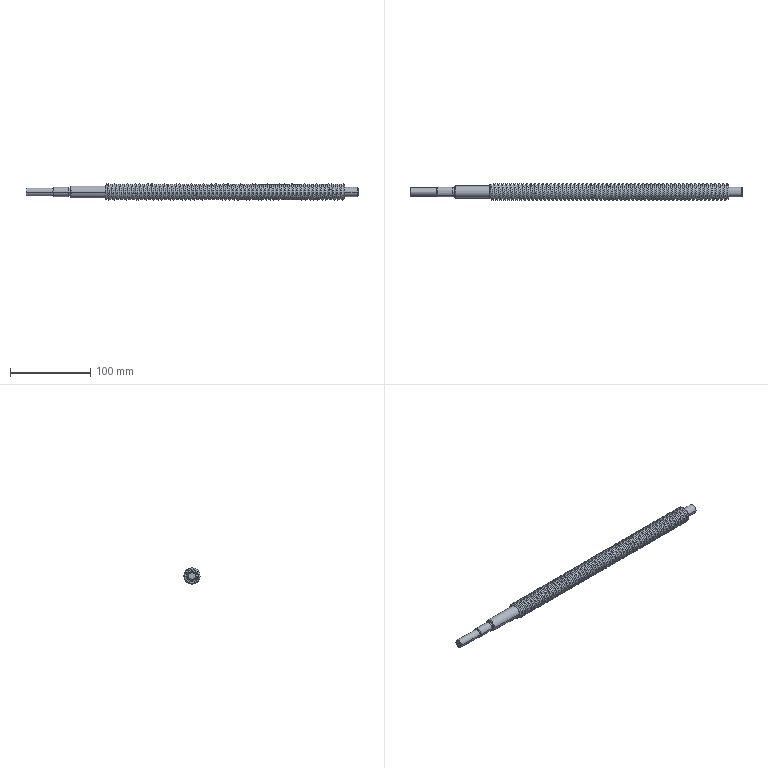Part | Creo | features DATUM PLANE 3, COORDINATE SYSTEM 1, CURVE 1, CUT 1, PROTRUSION 1 | 1 solid | 160 faces | box 414 x 20.009 x 20.003 mm | volume 92779 mm3 | cylinder 128 | spline 16 | cone 10 | plane 6 | commonest cylinder face diameters 20 x118 10 x4 11.667 x4 15 x2